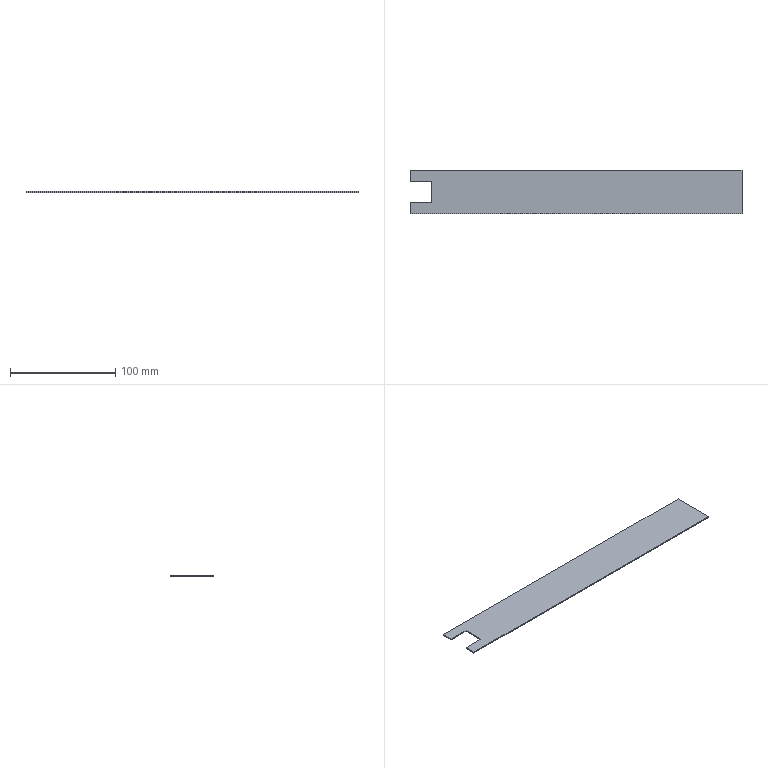Part | STEP file | Acrylic cover plate | 1 solid | 10 faces | box 315 x 41 x 1 mm | volume 12515 mm3 | plane 10
STEP:
#1=CARTESIAN_POINT('',(-125.,45.5,0.));
#2=VERTEX_POINT('',#1);
#3=CARTESIAN_POINT('',(-125.,35.,0.));
#4=VERTEX_POINT('',#3);
#5=CARTESIAN_POINT('',(-125.,45.5,0.));
#6=DIRECTION('',(0.,-1.,0.));
#7=VECTOR('',#6,1000.);
#8=LINE('',#5,#7);
#9=EDGE_CURVE('',#2,#4,#8,.T.);
#10=ORIENTED_EDGE('',*,*,#9,.T.);
#11=CARTESIAN_POINT('',(-125.,35.,1.));
#12=VERTEX_POINT('',#11);
#13=CARTESIAN_POINT('',(-125.,35.,-0.001));
#14=DIRECTION('',(0.,0.,1.));
#15=VECTOR('',#14,1000.);
#16=LINE('',#13,#15);
#17=EDGE_CURVE('',#4,#12,#16,.T.);
#18=ORIENTED_EDGE('',*,*,#17,.T.);
#19=CARTESIAN_POINT('',(-125.,45.5,1.));
#20=VERTEX_POINT('',#19);
#21=CARTESIAN_POINT('',(-125.,45.5,1.));
#22=DIRECTION('',(0.,-1.,0.));
#23=VECTOR('',#22,1000.);
#24=LINE('',#21,#23);
#25=EDGE_CURVE('',#20,#12,#24,.T.);
#26=ORIENTED_EDGE('',*,*,#25,.F.);
#27=CARTESIAN_POINT('',(-125.,45.5,1.));
#28=DIRECTION('',(0.,0.,-1.));
#29=VECTOR('',#28,1000.);
#30=LINE('',#27,#29);
#31=EDGE_CURVE('',#20,#2,#30,.T.);
#32=ORIENTED_EDGE('',*,*,#31,.T.);
#33=EDGE_LOOP('',(#10,#18,#26,#32));
#34=FACE_OUTER_BOUND('',#33,.T.);
#35=CARTESIAN_POINT('',(-125.,45.5,1.));
#36=DIRECTION('',(1.,0.,0.));
#37=DIRECTION('',(0.,1.,0.));
#38=AXIS2_PLACEMENT_3D('',#35,#36,#37);
#39=PLANE('',#38);
#40=ADVANCED_FACE('',(#34),#39,.F.);
#41=CARTESIAN_POINT('',(190.,4.5,0.));
#42=VERTEX_POINT('',#41);
#43=CARTESIAN_POINT('',(190.,45.5,0.));
#44=VERTEX_POINT('',#43);
#45=CARTESIAN_POINT('',(190.,45.5,0.));
#46=DIRECTION('',(0.,1.,0.));
#47=VECTOR('',#46,1000.);
#48=LINE('',#45,#47);
#49=EDGE_CURVE('',#42,#44,#48,.T.);
#50=ORIENTED_EDGE('',*,*,#49,.T.);
#51=CARTESIAN_POINT('',(190.,45.5,1.));
#52=VERTEX_POINT('',#51);
#53=CARTESIAN_POINT('',(190.,45.5,1.));
#54=DIRECTION('',(0.,0.,-1.));
#55=VECTOR('',#54,1000.);
#56=LINE('',#53,#55);
#57=EDGE_CURVE('',#52,#44,#56,.T.);
#58=ORIENTED_EDGE('',*,*,#57,.F.);
#59=CARTESIAN_POINT('',(190.,4.5,1.));
#60=VERTEX_POINT('',#59);
#61=CARTESIAN_POINT('',(190.,45.5,1.));
#62=DIRECTION('',(0.,1.,0.));
#63=VECTOR('',#62,1000.);
#64=LINE('',#61,#63);
#65=EDGE_CURVE('',#60,#52,#64,.T.);
#66=ORIENTED_EDGE('',*,*,#65,.F.);
#67=CARTESIAN_POINT('',(190.,4.5,1.));
#68=DIRECTION('',(0.,0.,-1.));
#69=VECTOR('',#68,1000.);
#70=LINE('',#67,#69);
#71=EDGE_CURVE('',#60,#42,#70,.T.);
#72=ORIENTED_EDGE('',*,*,#71,.T.);
#73=EDGE_LOOP('',(#50,#58,#66,#72));
#74=FACE_OUTER_BOUND('',#73,.T.);
#75=CARTESIAN_POINT('',(190.,45.5,1.));
#76=DIRECTION('',(-1.,0.,0.));
#77=DIRECTION('',(0.,0.,1.));
#78=AXIS2_PLACEMENT_3D('',#75,#76,#77);
#79=PLANE('',#78);
#80=ADVANCED_FACE('',(#74),#79,.F.);
#81=CARTESIAN_POINT('',(190.,45.5,0.));
#82=DIRECTION('',(-1.,0.,0.));
#83=VECTOR('',#82,1000.);
#84=LINE('',#81,#83);
#85=EDGE_CURVE('',#44,#2,#84,.T.);
#86=ORIENTED_EDGE('',*,*,#85,.T.);
#87=ORIENTED_EDGE('',*,*,#31,.F.);
#88=CARTESIAN_POINT('',(190.,45.5,1.));
#89=DIRECTION('',(-1.,0.,0.));
#90=VECTOR('',#89,1000.);
#91=LINE('',#88,#90);
#92=EDGE_CURVE('',#52,#20,#91,.T.);
#93=ORIENTED_EDGE('',*,*,#92,.F.);
#94=ORIENTED_EDGE('',*,*,#57,.T.);
#95=EDGE_LOOP('',(#86,#87,#93,#94));
#96=FACE_OUTER_BOUND('',#95,.T.);
#97=CARTESIAN_POINT('',(190.,45.5,1.));
#98=DIRECTION('',(0.,-1.,0.));
#99=DIRECTION('',(1.,0.,0.));
#100=AXIS2_PLACEMENT_3D('',#97,#98,#99);
#101=PLANE('',#100);
#102=ADVANCED_FACE('',(#96),#101,.F.);
#103=CARTESIAN_POINT('',(-125.,15.,1.));
#104=VERTEX_POINT('',#103);
#105=CARTESIAN_POINT('',(-125.,4.5,1.));
#106=VERTEX_POINT('',#105);
#107=CARTESIAN_POINT('',(-125.,45.5,1.));
#108=DIRECTION('',(0.,-1.,0.));
#109=VECTOR('',#108,1000.);
#110=LINE('',#107,#109);
#111=EDGE_CURVE('',#104,#106,#110,.T.);
#112=ORIENTED_EDGE('',*,*,#111,.F.);
#113=CARTESIAN_POINT('',(-125.,15.,0.));
#114=VERTEX_POINT('',#113);
#115=CARTESIAN_POINT('',(-125.,15.,-0.001));
#116=DIRECTION('',(0.,0.,1.));
#117=VECTOR('',#116,1000.);
#118=LINE('',#115,#117);
#119=EDGE_CURVE('',#114,#104,#118,.T.);
#120=ORIENTED_EDGE('',*,*,#119,.F.);
#121=CARTESIAN_POINT('',(-125.,4.5,0.));
#122=VERTEX_POINT('',#121);
#123=CARTESIAN_POINT('',(-125.,45.5,0.));
#124=DIRECTION('',(0.,-1.,0.));
#125=VECTOR('',#124,1000.);
#126=LINE('',#123,#125);
#127=EDGE_CURVE('',#114,#122,#126,.T.);
#128=ORIENTED_EDGE('',*,*,#127,.T.);
#129=CARTESIAN_POINT('',(-125.,4.5,1.));
#130=DIRECTION('',(0.,0.,-1.));
#131=VECTOR('',#130,1000.);
#132=LINE('',#129,#131);
#133=EDGE_CURVE('',#106,#122,#132,.T.);
#134=ORIENTED_EDGE('',*,*,#133,.F.);
#135=EDGE_LOOP('',(#112,#120,#128,#134));
#136=FACE_OUTER_BOUND('',#135,.T.);
#137=CARTESIAN_POINT('',(-125.,45.5,1.));
#138=DIRECTION('',(1.,0.,0.));
#139=DIRECTION('',(0.,1.,0.));
#140=AXIS2_PLACEMENT_3D('',#137,#138,#139);
#141=PLANE('',#140);
#142=ADVANCED_FACE('',(#136),#141,.F.);
#143=CARTESIAN_POINT('',(190.,4.5,0.));
#144=DIRECTION('',(1.,0.,0.));
#145=VECTOR('',#144,1000.);
#146=LINE('',#143,#145);
#147=EDGE_CURVE('',#122,#42,#146,.T.);
#148=ORIENTED_EDGE('',*,*,#147,.T.);
#149=ORIENTED_EDGE('',*,*,#71,.F.);
#150=CARTESIAN_POINT('',(190.,4.5,1.));
#151=DIRECTION('',(1.,0.,0.));
#152=VECTOR('',#151,1000.);
#153=LINE('',#150,#152);
#154=EDGE_CURVE('',#106,#60,#153,.T.);
#155=ORIENTED_EDGE('',*,*,#154,.F.);
#156=ORIENTED_EDGE('',*,*,#133,.T.);
#157=EDGE_LOOP('',(#148,#149,#155,#156));
#158=FACE_OUTER_BOUND('',#157,.T.);
#159=CARTESIAN_POINT('',(190.,4.5,1.));
#160=DIRECTION('',(0.,1.,0.));
#161=DIRECTION('',(-1.,0.,0.));
#162=AXIS2_PLACEMENT_3D('',#159,#160,#161);
#163=PLANE('',#162);
#164=ADVANCED_FACE('',(#158),#163,.F.);
#165=ORIENTED_EDGE('',*,*,#25,.T.);
#166=CARTESIAN_POINT('',(-105.,35.,1.));
#167=VERTEX_POINT('',#166);
#168=CARTESIAN_POINT('',(-125.,35.,1.));
#169=DIRECTION('',(-1.,0.,0.));
#170=VECTOR('',#169,1000.);
#171=LINE('',#168,#170);
#172=EDGE_CURVE('',#167,#12,#171,.T.);
#173=ORIENTED_EDGE('',*,*,#172,.F.);
#174=CARTESIAN_POINT('',(-105.,15.,1.));
#175=VERTEX_POINT('',#174);
#176=CARTESIAN_POINT('',(-105.,15.,1.));
#177=DIRECTION('',(0.,1.,0.));
#178=VECTOR('',#177,1000.);
#179=LINE('',#176,#178);
#180=EDGE_CURVE('',#175,#167,#179,.T.);
#181=ORIENTED_EDGE('',*,*,#180,.F.);
#182=CARTESIAN_POINT('',(-125.,15.,1.));
#183=DIRECTION('',(1.,0.,0.));
#184=VECTOR('',#183,1000.);
#185=LINE('',#182,#184);
#186=EDGE_CURVE('',#104,#175,#185,.T.);
#187=ORIENTED_EDGE('',*,*,#186,.F.);
#188=ORIENTED_EDGE('',*,*,#111,.T.);
#189=ORIENTED_EDGE('',*,*,#154,.T.);
#190=ORIENTED_EDGE('',*,*,#65,.T.);
#191=ORIENTED_EDGE('',*,*,#92,.T.);
#192=EDGE_LOOP('',(#165,#173,#181,#187,#188,#189,#190,#191));
#193=FACE_OUTER_BOUND('',#192,.T.);
#194=CARTESIAN_POINT('',(0.,0.,1.));
#195=DIRECTION('',(0.,0.,-1.));
#196=DIRECTION('',(-1.,0.,0.));
#197=AXIS2_PLACEMENT_3D('',#194,#195,#196);
#198=PLANE('',#197);
#199=ADVANCED_FACE('',(#193),#198,.F.);
#200=CARTESIAN_POINT('',(-105.,35.,0.));
#201=VERTEX_POINT('',#200);
#202=CARTESIAN_POINT('',(-125.,35.,0.));
#203=DIRECTION('',(-1.,0.,0.));
#204=VECTOR('',#203,1000.);
#205=LINE('',#202,#204);
#206=EDGE_CURVE('',#201,#4,#205,.T.);
#207=ORIENTED_EDGE('',*,*,#206,.T.);
#208=ORIENTED_EDGE('',*,*,#9,.F.);
#209=ORIENTED_EDGE('',*,*,#85,.F.);
#210=ORIENTED_EDGE('',*,*,#49,.F.);
#211=ORIENTED_EDGE('',*,*,#147,.F.);
#212=ORIENTED_EDGE('',*,*,#127,.F.);
#213=CARTESIAN_POINT('',(-105.,15.,0.));
#214=VERTEX_POINT('',#213);
#215=CARTESIAN_POINT('',(-125.,15.,0.));
#216=DIRECTION('',(1.,0.,0.));
#217=VECTOR('',#216,1000.);
#218=LINE('',#215,#217);
#219=EDGE_CURVE('',#114,#214,#218,.T.);
#220=ORIENTED_EDGE('',*,*,#219,.T.);
#221=CARTESIAN_POINT('',(-105.,15.,0.));
#222=DIRECTION('',(0.,1.,0.));
#223=VECTOR('',#222,1000.);
#224=LINE('',#221,#223);
#225=EDGE_CURVE('',#214,#201,#224,.T.);
#226=ORIENTED_EDGE('',*,*,#225,.T.);
#227=EDGE_LOOP('',(#207,#208,#209,#210,#211,#212,#220,#226));
#228=FACE_OUTER_BOUND('',#227,.T.);
#229=CARTESIAN_POINT('',(0.,0.,0.));
#230=DIRECTION('',(0.,0.,-1.));
#231=DIRECTION('',(-1.,0.,0.));
#232=AXIS2_PLACEMENT_3D('',#229,#230,#231);
#233=PLANE('',#232);
#234=ADVANCED_FACE('',(#228),#233,.T.);
#235=CARTESIAN_POINT('',(-105.,35.,-0.001));
#236=DIRECTION('',(0.,0.,1.));
#237=VECTOR('',#236,1000.);
#238=LINE('',#235,#237);
#239=EDGE_CURVE('',#201,#167,#238,.T.);
#240=ORIENTED_EDGE('',*,*,#239,.T.);
#241=ORIENTED_EDGE('',*,*,#172,.T.);
#242=ORIENTED_EDGE('',*,*,#17,.F.);
#243=ORIENTED_EDGE('',*,*,#206,.F.);
#244=EDGE_LOOP('',(#240,#241,#242,#243));
#245=FACE_OUTER_BOUND('',#244,.T.);
#246=CARTESIAN_POINT('',(-125.,35.,-0.001));
#247=DIRECTION('',(0.,1.,0.));
#248=DIRECTION('',(0.,0.,1.));
#249=AXIS2_PLACEMENT_3D('',#246,#247,#248);
#250=PLANE('',#249);
#251=ADVANCED_FACE('',(#245),#250,.F.);
#252=CARTESIAN_POINT('',(-105.,15.,-0.001));
#253=DIRECTION('',(0.,0.,1.));
#254=VECTOR('',#253,1000.);
#255=LINE('',#252,#254);
#256=EDGE_CURVE('',#214,#175,#255,.T.);
#257=ORIENTED_EDGE('',*,*,#256,.T.);
#258=ORIENTED_EDGE('',*,*,#180,.T.);
#259=ORIENTED_EDGE('',*,*,#239,.F.);
#260=ORIENTED_EDGE('',*,*,#225,.F.);
#261=EDGE_LOOP('',(#257,#258,#259,#260));
#262=FACE_OUTER_BOUND('',#261,.T.);
#263=CARTESIAN_POINT('',(-105.,15.,-0.001));
#264=DIRECTION('',(1.,0.,0.));
#265=DIRECTION('',(0.,0.,-1.));
#266=AXIS2_PLACEMENT_3D('',#263,#264,#265);
#267=PLANE('',#266);
#268=ADVANCED_FACE('',(#262),#267,.F.);
#269=ORIENTED_EDGE('',*,*,#119,.T.);
#270=ORIENTED_EDGE('',*,*,#186,.T.);
#271=ORIENTED_EDGE('',*,*,#256,.F.);
#272=ORIENTED_EDGE('',*,*,#219,.F.);
#273=EDGE_LOOP('',(#269,#270,#271,#272));
#274=FACE_OUTER_BOUND('',#273,.T.);
#275=CARTESIAN_POINT('',(-125.,15.,-0.001));
#276=DIRECTION('',(0.,-1.,0.));
#277=DIRECTION('',(0.,0.,-1.));
#278=AXIS2_PLACEMENT_3D('',#275,#276,#277);
#279=PLANE('',#278);
#280=ADVANCED_FACE('',(#274),#279,.F.);
#281=CLOSED_SHELL('',(#40,#80,#102,#142,#164,#199,#234,#251,#268,#280));
#282=MANIFOLD_SOLID_BREP('',#281);
#283=CARTESIAN_POINT('',(0.,0.,0.));
#284=DIRECTION('',(0.,0.,1.));
#285=DIRECTION('',(1.,0.,0.));
#286=AXIS2_PLACEMENT_3D('',#283,#284,#285);
#287=(LENGTH_UNIT()NAMED_UNIT(*)SI_UNIT(.MILLI.,.METRE.));
#288=UNCERTAINTY_MEASURE_WITH_UNIT(LENGTH_MEASURE(0.00001),#287,'','');
#289=(NAMED_UNIT(*)PLANE_ANGLE_UNIT()SI_UNIT($,.RADIAN.));
#290=(NAMED_UNIT(*)SI_UNIT($,.STERADIAN.)SOLID_ANGLE_UNIT());
#291=(GEOMETRIC_REPRESENTATION_CONTEXT(3)GLOBAL_UNCERTAINTY_ASSIGNED_CONTEXT((#288))GLOBAL_UNIT_ASSIGNED_CONTEXT((#287,#289,#290))REPRESENTATION_CONTEXT('',''));
#292=ADVANCED_BREP_SHAPE_REPRESENTATION('',(#282,#286),#291);